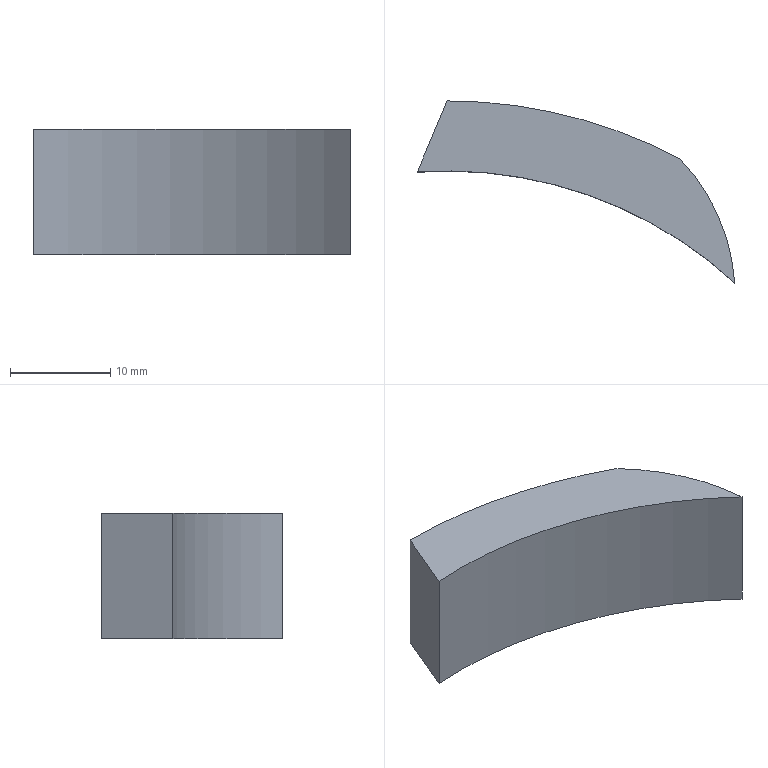Part | SolidWorks | features BaseBody 1 | 1 solid | 6 faces | box 31.73 x 18.182 x 12.5 mm | volume 2669 mm3 | cylinder 3 | plane 3 | commonest cylinder face diameters 40 x1 85 x1 99 x1
STEP:
#1=CARTESIAN_POINT('',(28.73,31.318,6.25));
#2=VERTEX_POINT('',#1);
#3=CARTESIAN_POINT('',(28.73,31.318,-6.25));
#4=VERTEX_POINT('',#3);
#5=CARTESIAN_POINT('',(28.73,31.318,6.25));
#6=DIRECTION('',(0.,0.,-1.));
#7=VECTOR('',#6,1000.);
#8=LINE('',#5,#7);
#9=EDGE_CURVE('',#2,#4,#8,.T.);
#10=ORIENTED_EDGE('',*,*,#9,.F.);
#11=CARTESIAN_POINT('',(-3.,42.394,6.25));
#12=VERTEX_POINT('',#11);
#13=CARTESIAN_POINT('',(0.,0.,6.25));
#14=DIRECTION('',(0.,0.,-1.));
#15=DIRECTION('',(-1.,0.,0.));
#16=AXIS2_PLACEMENT_3D('',#13,#14,#15);
#17=CIRCLE('',#16,42.5);
#18=EDGE_CURVE('',#12,#2,#17,.T.);
#19=ORIENTED_EDGE('',*,*,#18,.F.);
#20=CARTESIAN_POINT('',(-3.,42.394,-6.25));
#21=VERTEX_POINT('',#20);
#22=CARTESIAN_POINT('',(-3.,42.394,6.25));
#23=DIRECTION('',(0.,0.,1.));
#24=VECTOR('',#23,1000.);
#25=LINE('',#22,#24);
#26=EDGE_CURVE('',#21,#12,#25,.T.);
#27=ORIENTED_EDGE('',*,*,#26,.F.);
#28=CARTESIAN_POINT('',(0.,0.,-6.25));
#29=DIRECTION('',(0.,0.,1.));
#30=DIRECTION('',(-1.,0.,0.));
#31=AXIS2_PLACEMENT_3D('',#28,#29,#30);
#32=CIRCLE('',#31,42.5);
#33=EDGE_CURVE('',#4,#21,#32,.T.);
#34=ORIENTED_EDGE('',*,*,#33,.F.);
#35=EDGE_LOOP('',(#10,#19,#27,#34));
#36=FACE_OUTER_BOUND('',#35,.T.);
#37=CARTESIAN_POINT('',(0.,0.,6.25));
#38=DIRECTION('',(0.,0.,-1.));
#39=DIRECTION('',(-1.,0.,0.));
#40=AXIS2_PLACEMENT_3D('',#37,#38,#39);
#41=CYLINDRICAL_SURFACE('',#40,42.5);
#42=ADVANCED_FACE('',(#36),#41,.F.);
#43=CARTESIAN_POINT('',(23.284,43.682,-6.25));
#44=VERTEX_POINT('',#43);
#45=CARTESIAN_POINT('',(8.78,29.911,-6.25));
#46=DIRECTION('',(0.,0.,1.));
#47=DIRECTION('',(-1.,0.,0.));
#48=AXIS2_PLACEMENT_3D('',#45,#46,#47);
#49=CIRCLE('',#48,20.);
#50=EDGE_CURVE('',#4,#44,#49,.T.);
#51=ORIENTED_EDGE('',*,*,#50,.F.);
#52=ORIENTED_EDGE('',*,*,#33,.T.);
#53=CARTESIAN_POINT('',(0.,49.5,-6.25));
#54=VERTEX_POINT('',#53);
#55=CARTESIAN_POINT('',(0.,49.5,-6.25));
#56=DIRECTION('',(-0.3889,-0.9213,0.));
#57=VECTOR('',#56,1000.);
#58=LINE('',#55,#57);
#59=EDGE_CURVE('',#54,#21,#58,.T.);
#60=ORIENTED_EDGE('',*,*,#59,.F.);
#61=CARTESIAN_POINT('',(0.,0.,-6.25));
#62=DIRECTION('',(0.,0.,1.));
#63=DIRECTION('',(-1.,0.,0.));
#64=AXIS2_PLACEMENT_3D('',#61,#62,#63);
#65=CIRCLE('',#64,49.5);
#66=EDGE_CURVE('',#44,#54,#65,.T.);
#67=ORIENTED_EDGE('',*,*,#66,.F.);
#68=EDGE_LOOP('',(#51,#52,#60,#67));
#69=FACE_OUTER_BOUND('',#68,.T.);
#70=CARTESIAN_POINT('',(0.,0.,-6.25));
#71=DIRECTION('',(0.,0.,1.));
#72=DIRECTION('',(1.,0.,0.));
#73=AXIS2_PLACEMENT_3D('',#70,#71,#72);
#74=PLANE('',#73);
#75=ADVANCED_FACE('',(#69),#74,.F.);
#76=CARTESIAN_POINT('',(23.284,43.682,6.25));
#77=VERTEX_POINT('',#76);
#78=CARTESIAN_POINT('',(8.78,29.911,6.25));
#79=DIRECTION('',(0.,0.,-1.));
#80=DIRECTION('',(-1.,0.,0.));
#81=AXIS2_PLACEMENT_3D('',#78,#79,#80);
#82=CIRCLE('',#81,20.);
#83=EDGE_CURVE('',#77,#2,#82,.T.);
#84=ORIENTED_EDGE('',*,*,#83,.T.);
#85=ORIENTED_EDGE('',*,*,#9,.T.);
#86=ORIENTED_EDGE('',*,*,#50,.T.);
#87=CARTESIAN_POINT('',(23.284,43.682,6.25));
#88=DIRECTION('',(0.,0.,1.));
#89=VECTOR('',#88,1000.);
#90=LINE('',#87,#89);
#91=EDGE_CURVE('',#44,#77,#90,.T.);
#92=ORIENTED_EDGE('',*,*,#91,.T.);
#93=EDGE_LOOP('',(#84,#85,#86,#92));
#94=FACE_OUTER_BOUND('',#93,.T.);
#95=CARTESIAN_POINT('',(8.78,29.911,6.25));
#96=DIRECTION('',(0.,0.,-1.));
#97=DIRECTION('',(-1.,0.,0.));
#98=AXIS2_PLACEMENT_3D('',#95,#96,#97);
#99=CYLINDRICAL_SURFACE('',#98,20.);
#100=ADVANCED_FACE('',(#94),#99,.T.);
#101=ORIENTED_EDGE('',*,*,#18,.T.);
#102=ORIENTED_EDGE('',*,*,#83,.F.);
#103=CARTESIAN_POINT('',(0.,49.5,6.25));
#104=VERTEX_POINT('',#103);
#105=CARTESIAN_POINT('',(0.,0.,6.25));
#106=DIRECTION('',(0.,0.,1.));
#107=DIRECTION('',(-1.,0.,0.));
#108=AXIS2_PLACEMENT_3D('',#105,#106,#107);
#109=CIRCLE('',#108,49.5);
#110=EDGE_CURVE('',#77,#104,#109,.T.);
#111=ORIENTED_EDGE('',*,*,#110,.T.);
#112=CARTESIAN_POINT('',(0.,49.5,6.25));
#113=DIRECTION('',(-0.3889,-0.9213,0.));
#114=VECTOR('',#113,1000.);
#115=LINE('',#112,#114);
#116=EDGE_CURVE('',#104,#12,#115,.T.);
#117=ORIENTED_EDGE('',*,*,#116,.T.);
#118=EDGE_LOOP('',(#101,#102,#111,#117));
#119=FACE_OUTER_BOUND('',#118,.T.);
#120=CARTESIAN_POINT('',(0.,0.,6.25));
#121=DIRECTION('',(0.,0.,1.));
#122=DIRECTION('',(1.,0.,0.));
#123=AXIS2_PLACEMENT_3D('',#120,#121,#122);
#124=PLANE('',#123);
#125=ADVANCED_FACE('',(#119),#124,.T.);
#126=ORIENTED_EDGE('',*,*,#26,.T.);
#127=ORIENTED_EDGE('',*,*,#116,.F.);
#128=CARTESIAN_POINT('',(0.,49.5,6.25));
#129=DIRECTION('',(0.,0.,1.));
#130=VECTOR('',#129,1000.);
#131=LINE('',#128,#130);
#132=EDGE_CURVE('',#54,#104,#131,.T.);
#133=ORIENTED_EDGE('',*,*,#132,.F.);
#134=ORIENTED_EDGE('',*,*,#59,.T.);
#135=EDGE_LOOP('',(#126,#127,#133,#134));
#136=FACE_OUTER_BOUND('',#135,.T.);
#137=CARTESIAN_POINT('',(0.,49.5,6.25));
#138=DIRECTION('',(0.9213,-0.3889,0.));
#139=DIRECTION('',(0.3889,0.9213,0.));
#140=AXIS2_PLACEMENT_3D('',#137,#138,#139);
#141=PLANE('',#140);
#142=ADVANCED_FACE('',(#136),#141,.F.);
#143=ORIENTED_EDGE('',*,*,#110,.F.);
#144=ORIENTED_EDGE('',*,*,#91,.F.);
#145=ORIENTED_EDGE('',*,*,#66,.T.);
#146=ORIENTED_EDGE('',*,*,#132,.T.);
#147=EDGE_LOOP('',(#143,#144,#145,#146));
#148=FACE_OUTER_BOUND('',#147,.T.);
#149=CARTESIAN_POINT('',(0.,0.,6.25));
#150=DIRECTION('',(0.,0.,-1.));
#151=DIRECTION('',(-1.,0.,0.));
#152=AXIS2_PLACEMENT_3D('',#149,#150,#151);
#153=CYLINDRICAL_SURFACE('',#152,49.5);
#154=ADVANCED_FACE('',(#148),#153,.T.);
#155=CLOSED_SHELL('',(#42,#75,#100,#125,#142,#154));
#156=MANIFOLD_SOLID_BREP('',#155);
#157=CARTESIAN_POINT('',(0.,0.,0.));
#158=DIRECTION('',(0.,0.,1.));
#159=DIRECTION('',(1.,0.,0.));
#160=AXIS2_PLACEMENT_3D('',#157,#158,#159);
#161=(LENGTH_UNIT()NAMED_UNIT(*)SI_UNIT(.MILLI.,.METRE.));
#162=UNCERTAINTY_MEASURE_WITH_UNIT(LENGTH_MEASURE(0.00001),#161,'','');
#163=(NAMED_UNIT(*)PLANE_ANGLE_UNIT()SI_UNIT($,.RADIAN.));
#164=(NAMED_UNIT(*)SI_UNIT($,.STERADIAN.)SOLID_ANGLE_UNIT());
#165=(GEOMETRIC_REPRESENTATION_CONTEXT(3)GLOBAL_UNCERTAINTY_ASSIGNED_CONTEXT((#162))GLOBAL_UNIT_ASSIGNED_CONTEXT((#161,#163,#164))REPRESENTATION_CONTEXT('',''));
#166=ADVANCED_BREP_SHAPE_REPRESENTATION('',(#156,#160),#165);